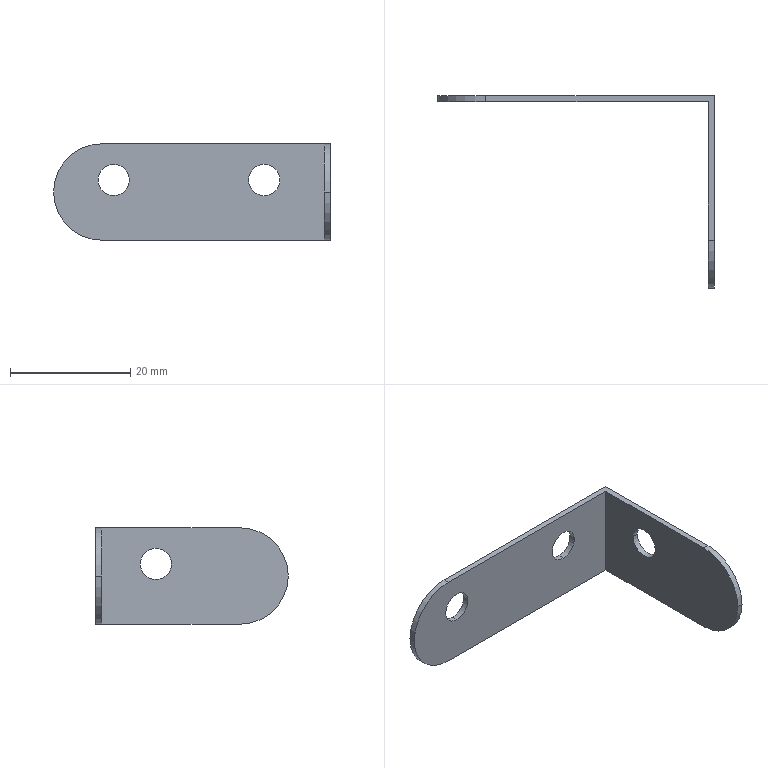Part | SolidWorks | features MirrorStock 1 | 1 solid | 16 faces | box 46 x 32 x 16 mm | volume 1113 mm3 | cylinder 10 | plane 6 | commonest cylinder face diameters 5.2 x6 16 x4
STEP:
#1=CARTESIAN_POINT('',(-1.,-7.4,2.));
#2=VERTEX_POINT('',#1);
#3=CARTESIAN_POINT('',(-1.,-12.6,2.));
#4=VERTEX_POINT('',#3);
#5=CARTESIAN_POINT('',(-1.,-10.,2.));
#6=DIRECTION('',(-1.,0.,0.));
#7=DIRECTION('',(0.,1.,0.));
#8=AXIS2_PLACEMENT_3D('',#5,#6,#7);
#9=CIRCLE('',#8,2.6);
#10=EDGE_CURVE('',#2,#4,#9,.T.);
#11=ORIENTED_EDGE('',*,*,#10,.T.);
#12=CARTESIAN_POINT('',(0.,-12.6,2.));
#13=VERTEX_POINT('',#12);
#14=CARTESIAN_POINT('',(-46.,-12.6,2.));
#15=DIRECTION('',(1.,0.,0.));
#16=VECTOR('',#15,1000.);
#17=LINE('',#14,#16);
#18=EDGE_CURVE('',#4,#13,#17,.T.);
#19=ORIENTED_EDGE('',*,*,#18,.T.);
#20=CARTESIAN_POINT('',(0.,-7.4,2.));
#21=VERTEX_POINT('',#20);
#22=CARTESIAN_POINT('',(0.,-10.,2.));
#23=DIRECTION('',(-1.,0.,0.));
#24=DIRECTION('',(0.,1.,0.));
#25=AXIS2_PLACEMENT_3D('',#22,#23,#24);
#26=CIRCLE('',#25,2.6);
#27=EDGE_CURVE('',#21,#13,#26,.T.);
#28=ORIENTED_EDGE('',*,*,#27,.F.);
#29=CARTESIAN_POINT('',(-46.,-7.4,2.));
#30=DIRECTION('',(1.,0.,0.));
#31=VECTOR('',#30,1000.);
#32=LINE('',#29,#31);
#33=EDGE_CURVE('',#2,#21,#32,.T.);
#34=ORIENTED_EDGE('',*,*,#33,.F.);
#35=EDGE_LOOP('',(#11,#19,#28,#34));
#36=FACE_OUTER_BOUND('',#35,.T.);
#37=CARTESIAN_POINT('',(-46.,-10.,2.));
#38=DIRECTION('',(1.,0.,0.));
#39=DIRECTION('',(0.,1.,0.));
#40=AXIS2_PLACEMENT_3D('',#37,#38,#39);
#41=CYLINDRICAL_SURFACE('',#40,2.6);
#42=ADVANCED_FACE('',(#36),#41,.F.);
#43=CARTESIAN_POINT('',(-36.,-1.,-0.6));
#44=VERTEX_POINT('',#43);
#45=CARTESIAN_POINT('',(-36.,-1.,4.6));
#46=VERTEX_POINT('',#45);
#47=CARTESIAN_POINT('',(-36.,-1.,2.));
#48=DIRECTION('',(0.,-1.,0.));
#49=DIRECTION('',(0.,0.,-1.));
#50=AXIS2_PLACEMENT_3D('',#47,#48,#49);
#51=CIRCLE('',#50,2.6);
#52=EDGE_CURVE('',#44,#46,#51,.T.);
#53=ORIENTED_EDGE('',*,*,#52,.T.);
#54=CARTESIAN_POINT('',(-36.,0.,4.6));
#55=VERTEX_POINT('',#54);
#56=CARTESIAN_POINT('',(-36.,-32.,4.6));
#57=DIRECTION('',(0.,1.,0.));
#58=VECTOR('',#57,1000.);
#59=LINE('',#56,#58);
#60=EDGE_CURVE('',#46,#55,#59,.T.);
#61=ORIENTED_EDGE('',*,*,#60,.T.);
#62=CARTESIAN_POINT('',(-36.,0.,-0.6));
#63=VERTEX_POINT('',#62);
#64=CARTESIAN_POINT('',(-36.,0.,2.));
#65=DIRECTION('',(0.,-1.,0.));
#66=DIRECTION('',(0.,0.,-1.));
#67=AXIS2_PLACEMENT_3D('',#64,#65,#66);
#68=CIRCLE('',#67,2.6);
#69=EDGE_CURVE('',#63,#55,#68,.T.);
#70=ORIENTED_EDGE('',*,*,#69,.F.);
#71=CARTESIAN_POINT('',(-36.,-32.,-0.6));
#72=DIRECTION('',(0.,1.,0.));
#73=VECTOR('',#72,1000.);
#74=LINE('',#71,#73);
#75=EDGE_CURVE('',#44,#63,#74,.T.);
#76=ORIENTED_EDGE('',*,*,#75,.F.);
#77=EDGE_LOOP('',(#53,#61,#70,#76));
#78=FACE_OUTER_BOUND('',#77,.T.);
#79=CARTESIAN_POINT('',(-36.,-32.,2.));
#80=DIRECTION('',(0.,1.,0.));
#81=DIRECTION('',(0.,0.,-1.));
#82=AXIS2_PLACEMENT_3D('',#79,#80,#81);
#83=CYLINDRICAL_SURFACE('',#82,2.6);
#84=ADVANCED_FACE('',(#78),#83,.F.);
#85=CARTESIAN_POINT('',(-11.,-1.,-0.6));
#86=VERTEX_POINT('',#85);
#87=CARTESIAN_POINT('',(-11.,-1.,4.6));
#88=VERTEX_POINT('',#87);
#89=CARTESIAN_POINT('',(-11.,-1.,2.));
#90=DIRECTION('',(0.,-1.,0.));
#91=DIRECTION('',(0.,0.,-1.));
#92=AXIS2_PLACEMENT_3D('',#89,#90,#91);
#93=CIRCLE('',#92,2.6);
#94=EDGE_CURVE('',#86,#88,#93,.T.);
#95=ORIENTED_EDGE('',*,*,#94,.T.);
#96=CARTESIAN_POINT('',(-11.,0.,4.6));
#97=VERTEX_POINT('',#96);
#98=CARTESIAN_POINT('',(-11.,-32.,4.6));
#99=DIRECTION('',(0.,1.,0.));
#100=VECTOR('',#99,1000.);
#101=LINE('',#98,#100);
#102=EDGE_CURVE('',#88,#97,#101,.T.);
#103=ORIENTED_EDGE('',*,*,#102,.T.);
#104=CARTESIAN_POINT('',(-11.,0.,-0.6));
#105=VERTEX_POINT('',#104);
#106=CARTESIAN_POINT('',(-11.,0.,2.));
#107=DIRECTION('',(0.,-1.,0.));
#108=DIRECTION('',(0.,0.,-1.));
#109=AXIS2_PLACEMENT_3D('',#106,#107,#108);
#110=CIRCLE('',#109,2.6);
#111=EDGE_CURVE('',#105,#97,#110,.T.);
#112=ORIENTED_EDGE('',*,*,#111,.F.);
#113=CARTESIAN_POINT('',(-11.,-32.,-0.6));
#114=DIRECTION('',(0.,1.,0.));
#115=VECTOR('',#114,1000.);
#116=LINE('',#113,#115);
#117=EDGE_CURVE('',#86,#105,#116,.T.);
#118=ORIENTED_EDGE('',*,*,#117,.F.);
#119=EDGE_LOOP('',(#95,#103,#112,#118));
#120=FACE_OUTER_BOUND('',#119,.T.);
#121=CARTESIAN_POINT('',(-11.,-32.,2.));
#122=DIRECTION('',(0.,1.,0.));
#123=DIRECTION('',(0.,0.,-1.));
#124=AXIS2_PLACEMENT_3D('',#121,#122,#123);
#125=CYLINDRICAL_SURFACE('',#124,2.6);
#126=ADVANCED_FACE('',(#120),#125,.F.);
#127=ORIENTED_EDGE('',*,*,#52,.F.);
#128=CARTESIAN_POINT('',(-36.,-1.,2.));
#129=DIRECTION('',(0.,-1.,0.));
#130=DIRECTION('',(0.,0.,-1.));
#131=AXIS2_PLACEMENT_3D('',#128,#129,#130);
#132=CIRCLE('',#131,2.6);
#133=EDGE_CURVE('',#46,#44,#132,.T.);
#134=ORIENTED_EDGE('',*,*,#133,.F.);
#135=EDGE_LOOP('',(#127,#134));
#136=FACE_BOUND('',#135,.T.);
#137=ORIENTED_EDGE('',*,*,#94,.F.);
#138=CARTESIAN_POINT('',(-11.,-1.,2.));
#139=DIRECTION('',(0.,-1.,0.));
#140=DIRECTION('',(0.,0.,-1.));
#141=AXIS2_PLACEMENT_3D('',#138,#139,#140);
#142=CIRCLE('',#141,2.6);
#143=EDGE_CURVE('',#88,#86,#142,.T.);
#144=ORIENTED_EDGE('',*,*,#143,.F.);
#145=EDGE_LOOP('',(#137,#144));
#146=FACE_BOUND('',#145,.T.);
#147=CARTESIAN_POINT('',(-38.,-1.,-8.));
#148=VERTEX_POINT('',#147);
#149=CARTESIAN_POINT('',(-1.,-1.,-8.));
#150=VERTEX_POINT('',#149);
#151=CARTESIAN_POINT('',(-46.,-1.,-8.));
#152=DIRECTION('',(1.,0.,0.));
#153=VECTOR('',#152,1000.);
#154=LINE('',#151,#153);
#155=EDGE_CURVE('',#148,#150,#154,.T.);
#156=ORIENTED_EDGE('',*,*,#155,.T.);
#157=CARTESIAN_POINT('',(-1.,-1.,8.));
#158=VERTEX_POINT('',#157);
#159=CARTESIAN_POINT('',(-1.,-1.,-8.));
#160=DIRECTION('',(0.,0.,1.));
#161=VECTOR('',#160,1000.);
#162=LINE('',#159,#161);
#163=EDGE_CURVE('',#150,#158,#162,.T.);
#164=ORIENTED_EDGE('',*,*,#163,.T.);
#165=CARTESIAN_POINT('',(-38.,-1.,8.));
#166=VERTEX_POINT('',#165);
#167=CARTESIAN_POINT('',(-46.,-1.,8.));
#168=DIRECTION('',(1.,0.,0.));
#169=VECTOR('',#168,1000.);
#170=LINE('',#167,#169);
#171=EDGE_CURVE('',#166,#158,#170,.T.);
#172=ORIENTED_EDGE('',*,*,#171,.F.);
#173=CARTESIAN_POINT('',(-46.,-1.,0.));
#174=VERTEX_POINT('',#173);
#175=CARTESIAN_POINT('',(-38.,-1.,0.));
#176=DIRECTION('',(0.,1.,0.));
#177=DIRECTION('',(0.,0.,-1.));
#178=AXIS2_PLACEMENT_3D('',#175,#176,#177);
#179=CIRCLE('',#178,8.);
#180=EDGE_CURVE('',#174,#166,#179,.T.);
#181=ORIENTED_EDGE('',*,*,#180,.F.);
#182=CARTESIAN_POINT('',(-38.,-1.,0.));
#183=DIRECTION('',(0.,1.,0.));
#184=DIRECTION('',(0.,0.,-1.));
#185=AXIS2_PLACEMENT_3D('',#182,#183,#184);
#186=CIRCLE('',#185,8.);
#187=EDGE_CURVE('',#148,#174,#186,.T.);
#188=ORIENTED_EDGE('',*,*,#187,.F.);
#189=EDGE_LOOP('',(#156,#164,#172,#181,#188));
#190=FACE_OUTER_BOUND('',#189,.T.);
#191=CARTESIAN_POINT('',(-46.,-1.,-8.));
#192=DIRECTION('',(0.,1.,0.));
#193=DIRECTION('',(0.,0.,-1.));
#194=AXIS2_PLACEMENT_3D('',#191,#192,#193);
#195=PLANE('',#194);
#196=ADVANCED_FACE('',(#136,#146,#190),#195,.F.);
#197=ORIENTED_EDGE('',*,*,#10,.F.);
#198=CARTESIAN_POINT('',(-1.,-10.,2.));
#199=DIRECTION('',(-1.,0.,0.));
#200=DIRECTION('',(0.,1.,0.));
#201=AXIS2_PLACEMENT_3D('',#198,#199,#200);
#202=CIRCLE('',#201,2.6);
#203=EDGE_CURVE('',#4,#2,#202,.T.);
#204=ORIENTED_EDGE('',*,*,#203,.F.);
#205=EDGE_LOOP('',(#197,#204));
#206=FACE_BOUND('',#205,.T.);
#207=CARTESIAN_POINT('',(-1.,-24.,8.));
#208=VERTEX_POINT('',#207);
#209=CARTESIAN_POINT('',(-1.,-32.,0.));
#210=VERTEX_POINT('',#209);
#211=CARTESIAN_POINT('',(-1.,-24.,0.));
#212=DIRECTION('',(1.,0.,0.));
#213=DIRECTION('',(0.,1.,0.));
#214=AXIS2_PLACEMENT_3D('',#211,#212,#213);
#215=CIRCLE('',#214,8.);
#216=EDGE_CURVE('',#208,#210,#215,.T.);
#217=ORIENTED_EDGE('',*,*,#216,.F.);
#218=CARTESIAN_POINT('',(-1.,-1.,8.));
#219=DIRECTION('',(0.,-1.,0.));
#220=VECTOR('',#219,1000.);
#221=LINE('',#218,#220);
#222=EDGE_CURVE('',#158,#208,#221,.T.);
#223=ORIENTED_EDGE('',*,*,#222,.F.);
#224=ORIENTED_EDGE('',*,*,#163,.F.);
#225=CARTESIAN_POINT('',(-1.,-24.,-8.));
#226=VERTEX_POINT('',#225);
#227=CARTESIAN_POINT('',(-1.,-1.,-8.));
#228=DIRECTION('',(0.,-1.,0.));
#229=VECTOR('',#228,1000.);
#230=LINE('',#227,#229);
#231=EDGE_CURVE('',#150,#226,#230,.T.);
#232=ORIENTED_EDGE('',*,*,#231,.T.);
#233=CARTESIAN_POINT('',(-1.,-24.,0.));
#234=DIRECTION('',(1.,0.,0.));
#235=DIRECTION('',(0.,1.,0.));
#236=AXIS2_PLACEMENT_3D('',#233,#234,#235);
#237=CIRCLE('',#236,8.);
#238=EDGE_CURVE('',#210,#226,#237,.T.);
#239=ORIENTED_EDGE('',*,*,#238,.F.);
#240=EDGE_LOOP('',(#217,#223,#224,#232,#239));
#241=FACE_OUTER_BOUND('',#240,.T.);
#242=CARTESIAN_POINT('',(-1.,-1.,-8.));
#243=DIRECTION('',(1.,0.,0.));
#244=DIRECTION('',(0.,1.,0.));
#245=AXIS2_PLACEMENT_3D('',#242,#243,#244);
#246=PLANE('',#245);
#247=ADVANCED_FACE('',(#206,#241),#246,.F.);
#248=ORIENTED_EDGE('',*,*,#27,.T.);
#249=CARTESIAN_POINT('',(0.,-10.,2.));
#250=DIRECTION('',(-1.,0.,0.));
#251=DIRECTION('',(0.,1.,0.));
#252=AXIS2_PLACEMENT_3D('',#249,#250,#251);
#253=CIRCLE('',#252,2.6);
#254=EDGE_CURVE('',#13,#21,#253,.T.);
#255=ORIENTED_EDGE('',*,*,#254,.T.);
#256=EDGE_LOOP('',(#248,#255));
#257=FACE_BOUND('',#256,.T.);
#258=CARTESIAN_POINT('',(0.,-24.,-8.));
#259=VERTEX_POINT('',#258);
#260=CARTESIAN_POINT('',(0.,0.,-8.));
#261=VERTEX_POINT('',#260);
#262=CARTESIAN_POINT('',(0.,0.,-8.));
#263=DIRECTION('',(0.,1.,0.));
#264=VECTOR('',#263,1000.);
#265=LINE('',#262,#264);
#266=EDGE_CURVE('',#259,#261,#265,.T.);
#267=ORIENTED_EDGE('',*,*,#266,.T.);
#268=CARTESIAN_POINT('',(0.,0.,8.));
#269=VERTEX_POINT('',#268);
#270=CARTESIAN_POINT('',(0.,0.,-8.));
#271=DIRECTION('',(0.,0.,1.));
#272=VECTOR('',#271,1000.);
#273=LINE('',#270,#272);
#274=EDGE_CURVE('',#261,#269,#273,.T.);
#275=ORIENTED_EDGE('',*,*,#274,.T.);
#276=CARTESIAN_POINT('',(0.,-24.,8.));
#277=VERTEX_POINT('',#276);
#278=CARTESIAN_POINT('',(0.,0.,8.));
#279=DIRECTION('',(0.,1.,0.));
#280=VECTOR('',#279,1000.);
#281=LINE('',#278,#280);
#282=EDGE_CURVE('',#277,#269,#281,.T.);
#283=ORIENTED_EDGE('',*,*,#282,.F.);
#284=CARTESIAN_POINT('',(0.,-32.,0.));
#285=VERTEX_POINT('',#284);
#286=CARTESIAN_POINT('',(0.,-24.,0.));
#287=DIRECTION('',(-1.,0.,0.));
#288=DIRECTION('',(0.,-1.,0.));
#289=AXIS2_PLACEMENT_3D('',#286,#287,#288);
#290=CIRCLE('',#289,8.);
#291=EDGE_CURVE('',#285,#277,#290,.T.);
#292=ORIENTED_EDGE('',*,*,#291,.F.);
#293=CARTESIAN_POINT('',(0.,-24.,0.));
#294=DIRECTION('',(-1.,0.,0.));
#295=DIRECTION('',(0.,-1.,0.));
#296=AXIS2_PLACEMENT_3D('',#293,#294,#295);
#297=CIRCLE('',#296,8.);
#298=EDGE_CURVE('',#259,#285,#297,.T.);
#299=ORIENTED_EDGE('',*,*,#298,.F.);
#300=EDGE_LOOP('',(#267,#275,#283,#292,#299));
#301=FACE_OUTER_BOUND('',#300,.T.);
#302=CARTESIAN_POINT('',(0.,0.,-8.));
#303=DIRECTION('',(-1.,0.,0.));
#304=DIRECTION('',(0.,-1.,0.));
#305=AXIS2_PLACEMENT_3D('',#302,#303,#304);
#306=PLANE('',#305);
#307=ADVANCED_FACE('',(#257,#301),#306,.F.);
#308=ORIENTED_EDGE('',*,*,#69,.T.);
#309=CARTESIAN_POINT('',(-36.,0.,2.));
#310=DIRECTION('',(0.,-1.,0.));
#311=DIRECTION('',(0.,0.,-1.));
#312=AXIS2_PLACEMENT_3D('',#309,#310,#311);
#313=CIRCLE('',#312,2.6);
#314=EDGE_CURVE('',#55,#63,#313,.T.);
#315=ORIENTED_EDGE('',*,*,#314,.T.);
#316=EDGE_LOOP('',(#308,#315));
#317=FACE_BOUND('',#316,.T.);
#318=ORIENTED_EDGE('',*,*,#111,.T.);
#319=CARTESIAN_POINT('',(-11.,0.,2.));
#320=DIRECTION('',(0.,-1.,0.));
#321=DIRECTION('',(0.,0.,-1.));
#322=AXIS2_PLACEMENT_3D('',#319,#320,#321);
#323=CIRCLE('',#322,2.6);
#324=EDGE_CURVE('',#97,#105,#323,.T.);
#325=ORIENTED_EDGE('',*,*,#324,.T.);
#326=EDGE_LOOP('',(#318,#325));
#327=FACE_BOUND('',#326,.T.);
#328=CARTESIAN_POINT('',(-38.,0.,8.));
#329=VERTEX_POINT('',#328);
#330=CARTESIAN_POINT('',(-46.,0.,0.));
#331=VERTEX_POINT('',#330);
#332=CARTESIAN_POINT('',(-38.,0.,0.));
#333=DIRECTION('',(0.,-1.,0.));
#334=DIRECTION('',(0.,0.,1.));
#335=AXIS2_PLACEMENT_3D('',#332,#333,#334);
#336=CIRCLE('',#335,8.);
#337=EDGE_CURVE('',#329,#331,#336,.T.);
#338=ORIENTED_EDGE('',*,*,#337,.F.);
#339=CARTESIAN_POINT('',(-46.,0.,8.));
#340=DIRECTION('',(-1.,0.,0.));
#341=VECTOR('',#340,1000.);
#342=LINE('',#339,#341);
#343=EDGE_CURVE('',#269,#329,#342,.T.);
#344=ORIENTED_EDGE('',*,*,#343,.F.);
#345=ORIENTED_EDGE('',*,*,#274,.F.);
#346=CARTESIAN_POINT('',(-38.,0.,-8.));
#347=VERTEX_POINT('',#346);
#348=CARTESIAN_POINT('',(-46.,0.,-8.));
#349=DIRECTION('',(-1.,0.,0.));
#350=VECTOR('',#349,1000.);
#351=LINE('',#348,#350);
#352=EDGE_CURVE('',#261,#347,#351,.T.);
#353=ORIENTED_EDGE('',*,*,#352,.T.);
#354=CARTESIAN_POINT('',(-38.,0.,0.));
#355=DIRECTION('',(0.,-1.,0.));
#356=DIRECTION('',(0.,0.,1.));
#357=AXIS2_PLACEMENT_3D('',#354,#355,#356);
#358=CIRCLE('',#357,8.);
#359=EDGE_CURVE('',#331,#347,#358,.T.);
#360=ORIENTED_EDGE('',*,*,#359,.F.);
#361=EDGE_LOOP('',(#338,#344,#345,#353,#360));
#362=FACE_OUTER_BOUND('',#361,.T.);
#363=CARTESIAN_POINT('',(-46.,0.,-8.));
#364=DIRECTION('',(0.,-1.,0.));
#365=DIRECTION('',(0.,0.,1.));
#366=AXIS2_PLACEMENT_3D('',#363,#364,#365);
#367=PLANE('',#366);
#368=ADVANCED_FACE('',(#317,#327,#362),#367,.F.);
#369=ORIENTED_EDGE('',*,*,#352,.F.);
#370=ORIENTED_EDGE('',*,*,#266,.F.);
#371=CARTESIAN_POINT('',(0.,-24.,-8.));
#372=DIRECTION('',(1.,0.,0.));
#373=VECTOR('',#372,1000.);
#374=LINE('',#371,#373);
#375=EDGE_CURVE('',#226,#259,#374,.T.);
#376=ORIENTED_EDGE('',*,*,#375,.F.);
#377=ORIENTED_EDGE('',*,*,#231,.F.);
#378=ORIENTED_EDGE('',*,*,#155,.F.);
#379=CARTESIAN_POINT('',(-38.,-1.,-8.));
#380=DIRECTION('',(0.,-1.,0.));
#381=VECTOR('',#380,1000.);
#382=LINE('',#379,#381);
#383=EDGE_CURVE('',#347,#148,#382,.T.);
#384=ORIENTED_EDGE('',*,*,#383,.F.);
#385=EDGE_LOOP('',(#369,#370,#376,#377,#378,#384));
#386=FACE_OUTER_BOUND('',#385,.T.);
#387=CARTESIAN_POINT('',(-46.,-1.,-8.));
#388=DIRECTION('',(0.,0.,-1.));
#389=DIRECTION('',(1.,0.,0.));
#390=AXIS2_PLACEMENT_3D('',#387,#388,#389);
#391=PLANE('',#390);
#392=ADVANCED_FACE('',(#386),#391,.T.);
#393=ORIENTED_EDGE('',*,*,#171,.T.);
#394=ORIENTED_EDGE('',*,*,#222,.T.);
#395=CARTESIAN_POINT('',(-46.,-24.,8.));
#396=DIRECTION('',(-1.,0.,0.));
#397=VECTOR('',#396,1000.);
#398=LINE('',#395,#397);
#399=EDGE_CURVE('',#277,#208,#398,.T.);
#400=ORIENTED_EDGE('',*,*,#399,.F.);
#401=ORIENTED_EDGE('',*,*,#282,.T.);
#402=ORIENTED_EDGE('',*,*,#343,.T.);
#403=CARTESIAN_POINT('',(-38.,-1.,8.));
#404=DIRECTION('',(0.,1.,0.));
#405=VECTOR('',#404,1000.);
#406=LINE('',#403,#405);
#407=EDGE_CURVE('',#166,#329,#406,.T.);
#408=ORIENTED_EDGE('',*,*,#407,.F.);
#409=EDGE_LOOP('',(#393,#394,#400,#401,#402,#408));
#410=FACE_OUTER_BOUND('',#409,.T.);
#411=CARTESIAN_POINT('',(-46.,-1.,8.));
#412=DIRECTION('',(0.,0.,-1.));
#413=DIRECTION('',(1.,0.,0.));
#414=AXIS2_PLACEMENT_3D('',#411,#412,#413);
#415=PLANE('',#414);
#416=ADVANCED_FACE('',(#410),#415,.F.);
#417=ORIENTED_EDGE('',*,*,#102,.F.);
#418=ORIENTED_EDGE('',*,*,#143,.T.);
#419=ORIENTED_EDGE('',*,*,#117,.T.);
#420=ORIENTED_EDGE('',*,*,#324,.F.);
#421=EDGE_LOOP('',(#417,#418,#419,#420));
#422=FACE_OUTER_BOUND('',#421,.T.);
#423=CARTESIAN_POINT('',(-11.,-32.,2.));
#424=DIRECTION('',(0.,1.,0.));
#425=DIRECTION('',(0.,0.,-1.));
#426=AXIS2_PLACEMENT_3D('',#423,#424,#425);
#427=CYLINDRICAL_SURFACE('',#426,2.6);
#428=ADVANCED_FACE('',(#422),#427,.F.);
#429=ORIENTED_EDGE('',*,*,#60,.F.);
#430=ORIENTED_EDGE('',*,*,#133,.T.);
#431=ORIENTED_EDGE('',*,*,#75,.T.);
#432=ORIENTED_EDGE('',*,*,#314,.F.);
#433=EDGE_LOOP('',(#429,#430,#431,#432));
#434=FACE_OUTER_BOUND('',#433,.T.);
#435=CARTESIAN_POINT('',(-36.,-32.,2.));
#436=DIRECTION('',(0.,1.,0.));
#437=DIRECTION('',(0.,0.,-1.));
#438=AXIS2_PLACEMENT_3D('',#435,#436,#437);
#439=CYLINDRICAL_SURFACE('',#438,2.6);
#440=ADVANCED_FACE('',(#434),#439,.F.);
#441=ORIENTED_EDGE('',*,*,#18,.F.);
#442=ORIENTED_EDGE('',*,*,#203,.T.);
#443=ORIENTED_EDGE('',*,*,#33,.T.);
#444=ORIENTED_EDGE('',*,*,#254,.F.);
#445=EDGE_LOOP('',(#441,#442,#443,#444));
#446=FACE_OUTER_BOUND('',#445,.T.);
#447=CARTESIAN_POINT('',(-46.,-10.,2.));
#448=DIRECTION('',(1.,0.,0.));
#449=DIRECTION('',(0.,1.,0.));
#450=AXIS2_PLACEMENT_3D('',#447,#448,#449);
#451=CYLINDRICAL_SURFACE('',#450,2.6);
#452=ADVANCED_FACE('',(#446),#451,.F.);
#453=CARTESIAN_POINT('',(-46.,0.,0.));
#454=DIRECTION('',(0.,-1.,0.));
#455=VECTOR('',#454,1000.);
#456=LINE('',#453,#455);
#457=EDGE_CURVE('',#331,#174,#456,.T.);
#458=ORIENTED_EDGE('',*,*,#457,.T.);
#459=ORIENTED_EDGE('',*,*,#180,.T.);
#460=ORIENTED_EDGE('',*,*,#407,.T.);
#461=ORIENTED_EDGE('',*,*,#337,.T.);
#462=EDGE_LOOP('',(#458,#459,#460,#461));
#463=FACE_OUTER_BOUND('',#462,.T.);
#464=CARTESIAN_POINT('',(-38.,0.,0.));
#465=DIRECTION('',(0.,-1.,0.));
#466=DIRECTION('',(0.,0.,1.));
#467=AXIS2_PLACEMENT_3D('',#464,#465,#466);
#468=CYLINDRICAL_SURFACE('',#467,8.);
#469=ADVANCED_FACE('',(#463),#468,.T.);
#470=ORIENTED_EDGE('',*,*,#359,.T.);
#471=ORIENTED_EDGE('',*,*,#383,.T.);
#472=ORIENTED_EDGE('',*,*,#187,.T.);
#473=ORIENTED_EDGE('',*,*,#457,.F.);
#474=EDGE_LOOP('',(#470,#471,#472,#473));
#475=FACE_OUTER_BOUND('',#474,.T.);
#476=CARTESIAN_POINT('',(-38.,-1.,0.));
#477=DIRECTION('',(0.,1.,0.));
#478=DIRECTION('',(0.,0.,-1.));
#479=AXIS2_PLACEMENT_3D('',#476,#477,#478);
#480=CYLINDRICAL_SURFACE('',#479,8.);
#481=ADVANCED_FACE('',(#475),#480,.T.);
#482=CARTESIAN_POINT('',(-1.,-32.,0.));
#483=DIRECTION('',(1.,0.,0.));
#484=VECTOR('',#483,1000.);
#485=LINE('',#482,#484);
#486=EDGE_CURVE('',#210,#285,#485,.T.);
#487=ORIENTED_EDGE('',*,*,#486,.T.);
#488=ORIENTED_EDGE('',*,*,#291,.T.);
#489=ORIENTED_EDGE('',*,*,#399,.T.);
#490=ORIENTED_EDGE('',*,*,#216,.T.);
#491=EDGE_LOOP('',(#487,#488,#489,#490));
#492=FACE_OUTER_BOUND('',#491,.T.);
#493=CARTESIAN_POINT('',(-1.,-24.,0.));
#494=DIRECTION('',(1.,0.,0.));
#495=DIRECTION('',(0.,0.,1.));
#496=AXIS2_PLACEMENT_3D('',#493,#494,#495);
#497=CYLINDRICAL_SURFACE('',#496,8.);
#498=ADVANCED_FACE('',(#492),#497,.T.);
#499=ORIENTED_EDGE('',*,*,#238,.T.);
#500=ORIENTED_EDGE('',*,*,#375,.T.);
#501=ORIENTED_EDGE('',*,*,#298,.T.);
#502=ORIENTED_EDGE('',*,*,#486,.F.);
#503=EDGE_LOOP('',(#499,#500,#501,#502));
#504=FACE_OUTER_BOUND('',#503,.T.);
#505=CARTESIAN_POINT('',(-46.,-24.,0.));
#506=DIRECTION('',(-1.,0.,0.));
#507=DIRECTION('',(0.,0.,-1.));
#508=AXIS2_PLACEMENT_3D('',#505,#506,#507);
#509=CYLINDRICAL_SURFACE('',#508,8.);
#510=ADVANCED_FACE('',(#504),#509,.T.);
#511=CLOSED_SHELL('',(#42,#84,#126,#196,#247,#307,#368,#392,#416,#428,#440,#452,#469,#481,#498,#510));
#512=MANIFOLD_SOLID_BREP('',#511);
#513=CARTESIAN_POINT('',(0.,0.,0.));
#514=DIRECTION('',(0.,0.,1.));
#515=DIRECTION('',(1.,0.,0.));
#516=AXIS2_PLACEMENT_3D('',#513,#514,#515);
#517=(LENGTH_UNIT()NAMED_UNIT(*)SI_UNIT(.MILLI.,.METRE.));
#518=UNCERTAINTY_MEASURE_WITH_UNIT(LENGTH_MEASURE(0.00001),#517,'','');
#519=(NAMED_UNIT(*)PLANE_ANGLE_UNIT()SI_UNIT($,.RADIAN.));
#520=(NAMED_UNIT(*)SI_UNIT($,.STERADIAN.)SOLID_ANGLE_UNIT());
#521=(GEOMETRIC_REPRESENTATION_CONTEXT(3)GLOBAL_UNCERTAINTY_ASSIGNED_CONTEXT((#518))GLOBAL_UNIT_ASSIGNED_CONTEXT((#517,#519,#520))REPRESENTATION_CONTEXT('',''));
#522=ADVANCED_BREP_SHAPE_REPRESENTATION('',(#512,#516),#521);